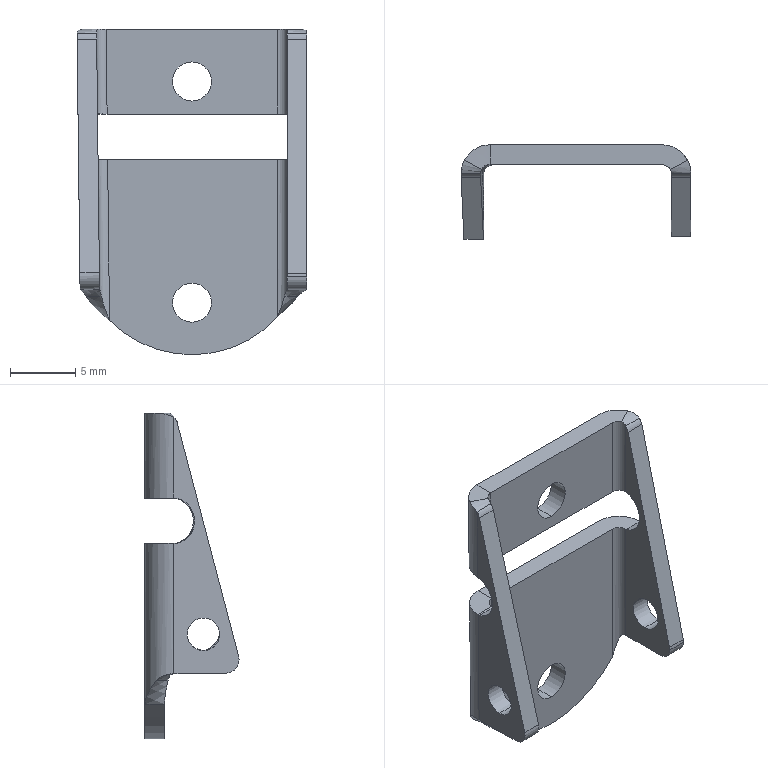Part | SolidWorks | features Fillet 3, HoleWzd 3, BaseBody 1 | 1 solid | 53 faces | box 17.668 x 7.243 x 25.011 mm | volume 631.719 mm3 | cylinder 26 | plane 17 | spline 10 | commonest cylinder face diameters 2.5 x6 2 x5 1.473 x4 3 x4 4.473 x4 3.572 x2